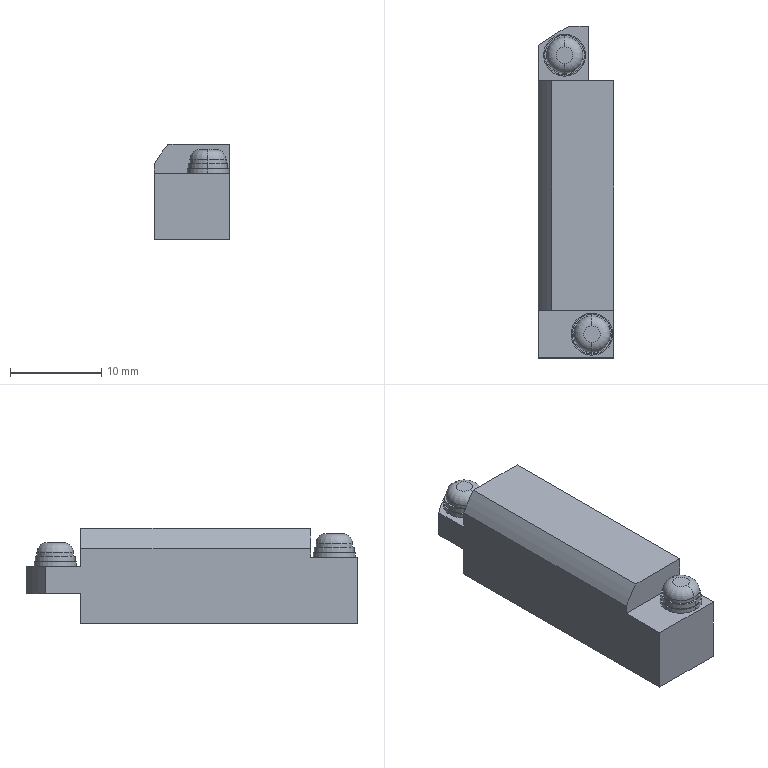Part | STEP file | Guide wheel mechanism revised.sldasm-Part-33 | 1 solid | 36 faces | box 8.3 x 36.4 x 10.5 mm | volume 2626 mm3 | plane 18 | cylinder 14 | torus 4 | commonest cylinder face diameters 4 x4 4.35 x4 4.6 x4 32 x1 47 x1
STEP:
#1=CARTESIAN_POINT('',(-8.1,318.9,-3.2));
#2=VERTEX_POINT('',#1);
#3=CARTESIAN_POINT('',(-8.1,323.5,-3.2));
#4=VERTEX_POINT('',#3);
#5=CARTESIAN_POINT('',(-8.1,321.2,-3.2));
#6=DIRECTION('',(0.,0.,1.));
#7=DIRECTION('',(0.,-1.,0.));
#8=AXIS2_PLACEMENT_3D('',#5,#6,#7);
#9=CIRCLE('',#8,2.3);
#10=EDGE_CURVE('',#2,#4,#9,.T.);
#11=ORIENTED_EDGE('',*,*,#10,.T.);
#12=CARTESIAN_POINT('',(-8.1,323.5,-2.7));
#13=VERTEX_POINT('',#12);
#14=CARTESIAN_POINT('',(-8.1,323.5,-0.6));
#15=DIRECTION('',(0.,0.,1.));
#16=VECTOR('',#15,1000.);
#17=LINE('',#14,#16);
#18=EDGE_CURVE('',#4,#13,#17,.T.);
#19=ORIENTED_EDGE('',*,*,#18,.T.);
#20=CARTESIAN_POINT('',(-8.1,318.9,-2.7));
#21=VERTEX_POINT('',#20);
#22=CARTESIAN_POINT('',(-8.1,321.2,-2.7));
#23=DIRECTION('',(0.,0.,-1.));
#24=DIRECTION('',(0.,-1.,0.));
#25=AXIS2_PLACEMENT_3D('',#22,#23,#24);
#26=CIRCLE('',#25,2.3);
#27=EDGE_CURVE('',#13,#21,#26,.T.);
#28=ORIENTED_EDGE('',*,*,#27,.T.);
#29=CARTESIAN_POINT('',(-8.1,318.9,-0.6));
#30=DIRECTION('',(0.,0.,1.));
#31=VECTOR('',#30,1000.);
#32=LINE('',#29,#31);
#33=EDGE_CURVE('',#2,#21,#32,.T.);
#34=ORIENTED_EDGE('',*,*,#33,.F.);
#35=EDGE_LOOP('',(#11,#19,#28,#34));
#36=FACE_OUTER_BOUND('',#35,.T.);
#37=CARTESIAN_POINT('',(-8.1,321.2,-0.6));
#38=DIRECTION('',(0.,0.,1.));
#39=DIRECTION('',(0.,-1.,0.));
#40=AXIS2_PLACEMENT_3D('',#37,#38,#39);
#41=CYLINDRICAL_SURFACE('',#40,2.3);
#42=ADVANCED_FACE('',(#36),#41,.T.);
#43=CARTESIAN_POINT('',(-11.1,354.1,-4.2));
#44=VERTEX_POINT('',#43);
#45=CARTESIAN_POINT('',(-11.1,349.5,-4.2));
#46=VERTEX_POINT('',#45);
#47=CARTESIAN_POINT('',(-11.1,351.8,-4.2));
#48=DIRECTION('',(0.,0.,-1.));
#49=DIRECTION('',(0.,-1.,0.));
#50=AXIS2_PLACEMENT_3D('',#47,#48,#49);
#51=CIRCLE('',#50,2.3);
#52=EDGE_CURVE('',#44,#46,#51,.T.);
#53=ORIENTED_EDGE('',*,*,#52,.F.);
#54=CARTESIAN_POINT('',(-11.1,354.1,-3.7));
#55=VERTEX_POINT('',#54);
#56=CARTESIAN_POINT('',(-11.1,354.1,-1.6));
#57=DIRECTION('',(0.,0.,1.));
#58=VECTOR('',#57,1000.);
#59=LINE('',#56,#58);
#60=EDGE_CURVE('',#44,#55,#59,.T.);
#61=ORIENTED_EDGE('',*,*,#60,.T.);
#62=CARTESIAN_POINT('',(-11.1,349.5,-3.7));
#63=VERTEX_POINT('',#62);
#64=CARTESIAN_POINT('',(-11.1,351.8,-3.7));
#65=DIRECTION('',(0.,0.,-1.));
#66=DIRECTION('',(0.,-1.,0.));
#67=AXIS2_PLACEMENT_3D('',#64,#65,#66);
#68=CIRCLE('',#67,2.3);
#69=EDGE_CURVE('',#55,#63,#68,.T.);
#70=ORIENTED_EDGE('',*,*,#69,.T.);
#71=CARTESIAN_POINT('',(-11.1,349.5,-1.6));
#72=DIRECTION('',(0.,0.,1.));
#73=VECTOR('',#72,1000.);
#74=LINE('',#71,#73);
#75=EDGE_CURVE('',#46,#63,#74,.T.);
#76=ORIENTED_EDGE('',*,*,#75,.F.);
#77=EDGE_LOOP('',(#53,#61,#70,#76));
#78=FACE_OUTER_BOUND('',#77,.T.);
#79=CARTESIAN_POINT('',(-11.1,351.8,-1.6));
#80=DIRECTION('',(0.,0.,1.));
#81=DIRECTION('',(0.,-1.,0.));
#82=AXIS2_PLACEMENT_3D('',#79,#80,#81);
#83=CYLINDRICAL_SURFACE('',#82,2.3);
#84=ADVANCED_FACE('',(#78),#83,.T.);
#85=CARTESIAN_POINT('',(-8.1,323.375,-2.7));
#86=VERTEX_POINT('',#85);
#87=CARTESIAN_POINT('',(-8.1,319.025,-2.7));
#88=VERTEX_POINT('',#87);
#89=CARTESIAN_POINT('',(-8.1,321.2,-2.7));
#90=DIRECTION('',(0.,0.,-1.));
#91=DIRECTION('',(0.,-1.,0.));
#92=AXIS2_PLACEMENT_3D('',#89,#90,#91);
#93=CIRCLE('',#92,2.175);
#94=EDGE_CURVE('',#86,#88,#93,.T.);
#95=ORIENTED_EDGE('',*,*,#94,.F.);
#96=CARTESIAN_POINT('',(-8.1,323.375,-2.1));
#97=VERTEX_POINT('',#96);
#98=CARTESIAN_POINT('',(-8.1,323.375,-0.6));
#99=DIRECTION('',(0.,0.,1.));
#100=VECTOR('',#99,1000.);
#101=LINE('',#98,#100);
#102=EDGE_CURVE('',#86,#97,#101,.T.);
#103=ORIENTED_EDGE('',*,*,#102,.T.);
#104=CARTESIAN_POINT('',(-8.1,319.025,-2.1));
#105=VERTEX_POINT('',#104);
#106=CARTESIAN_POINT('',(-8.1,321.2,-2.1));
#107=DIRECTION('',(0.,0.,-1.));
#108=DIRECTION('',(0.,-1.,0.));
#109=AXIS2_PLACEMENT_3D('',#106,#107,#108);
#110=CIRCLE('',#109,2.175);
#111=EDGE_CURVE('',#97,#105,#110,.T.);
#112=ORIENTED_EDGE('',*,*,#111,.T.);
#113=CARTESIAN_POINT('',(-8.1,319.025,-0.6));
#114=DIRECTION('',(0.,0.,1.));
#115=VECTOR('',#114,1000.);
#116=LINE('',#113,#115);
#117=EDGE_CURVE('',#88,#105,#116,.T.);
#118=ORIENTED_EDGE('',*,*,#117,.F.);
#119=EDGE_LOOP('',(#95,#103,#112,#118));
#120=FACE_OUTER_BOUND('',#119,.T.);
#121=CARTESIAN_POINT('',(-8.1,321.2,-0.6));
#122=DIRECTION('',(0.,0.,1.));
#123=DIRECTION('',(0.,-1.,0.));
#124=AXIS2_PLACEMENT_3D('',#121,#122,#123);
#125=CYLINDRICAL_SURFACE('',#124,2.175);
#126=ADVANCED_FACE('',(#120),#125,.T.);
#127=CARTESIAN_POINT('',(-11.1,349.625,-3.7));
#128=VERTEX_POINT('',#127);
#129=CARTESIAN_POINT('',(-11.1,353.975,-3.7));
#130=VERTEX_POINT('',#129);
#131=CARTESIAN_POINT('',(-11.1,351.8,-3.7));
#132=DIRECTION('',(0.,0.,1.));
#133=DIRECTION('',(0.,-1.,0.));
#134=AXIS2_PLACEMENT_3D('',#131,#132,#133);
#135=CIRCLE('',#134,2.175);
#136=EDGE_CURVE('',#128,#130,#135,.T.);
#137=ORIENTED_EDGE('',*,*,#136,.T.);
#138=CARTESIAN_POINT('',(-11.1,353.975,-3.1));
#139=VERTEX_POINT('',#138);
#140=CARTESIAN_POINT('',(-11.1,353.975,-1.6));
#141=DIRECTION('',(0.,0.,1.));
#142=VECTOR('',#141,1000.);
#143=LINE('',#140,#142);
#144=EDGE_CURVE('',#130,#139,#143,.T.);
#145=ORIENTED_EDGE('',*,*,#144,.T.);
#146=CARTESIAN_POINT('',(-11.1,349.625,-3.1));
#147=VERTEX_POINT('',#146);
#148=CARTESIAN_POINT('',(-11.1,351.8,-3.1));
#149=DIRECTION('',(0.,0.,-1.));
#150=DIRECTION('',(0.,-1.,0.));
#151=AXIS2_PLACEMENT_3D('',#148,#149,#150);
#152=CIRCLE('',#151,2.175);
#153=EDGE_CURVE('',#139,#147,#152,.T.);
#154=ORIENTED_EDGE('',*,*,#153,.T.);
#155=CARTESIAN_POINT('',(-11.1,349.625,-1.6));
#156=DIRECTION('',(0.,0.,1.));
#157=VECTOR('',#156,1000.);
#158=LINE('',#155,#157);
#159=EDGE_CURVE('',#128,#147,#158,.T.);
#160=ORIENTED_EDGE('',*,*,#159,.F.);
#161=EDGE_LOOP('',(#137,#145,#154,#160));
#162=FACE_OUTER_BOUND('',#161,.T.);
#163=CARTESIAN_POINT('',(-11.1,351.8,-1.6));
#164=DIRECTION('',(0.,0.,1.));
#165=DIRECTION('',(0.,-1.,0.));
#166=AXIS2_PLACEMENT_3D('',#163,#164,#165);
#167=CYLINDRICAL_SURFACE('',#166,2.175);
#168=ADVANCED_FACE('',(#162),#167,.T.);
#169=CARTESIAN_POINT('',(-8.1,323.2,-2.1));
#170=VERTEX_POINT('',#169);
#171=CARTESIAN_POINT('',(-8.1,319.2,-2.1));
#172=VERTEX_POINT('',#171);
#173=CARTESIAN_POINT('',(-8.1,321.2,-2.1));
#174=DIRECTION('',(0.,0.,-1.));
#175=DIRECTION('',(0.,-1.,0.));
#176=AXIS2_PLACEMENT_3D('',#173,#174,#175);
#177=CIRCLE('',#176,2.);
#178=EDGE_CURVE('',#170,#172,#177,.T.);
#179=ORIENTED_EDGE('',*,*,#178,.F.);
#180=CARTESIAN_POINT('',(-8.1,323.2,-1.7));
#181=VERTEX_POINT('',#180);
#182=CARTESIAN_POINT('',(-8.1,323.2,-0.6));
#183=DIRECTION('',(0.,0.,1.));
#184=VECTOR('',#183,1000.);
#185=LINE('',#182,#184);
#186=EDGE_CURVE('',#170,#181,#185,.T.);
#187=ORIENTED_EDGE('',*,*,#186,.T.);
#188=CARTESIAN_POINT('',(-8.1,319.2,-1.7));
#189=VERTEX_POINT('',#188);
#190=CARTESIAN_POINT('',(-8.1,321.2,-1.7));
#191=DIRECTION('',(0.,0.,-1.));
#192=DIRECTION('',(0.,-1.,0.));
#193=AXIS2_PLACEMENT_3D('',#190,#191,#192);
#194=CIRCLE('',#193,2.);
#195=EDGE_CURVE('',#181,#189,#194,.T.);
#196=ORIENTED_EDGE('',*,*,#195,.T.);
#197=CARTESIAN_POINT('',(-8.1,319.2,-0.6));
#198=DIRECTION('',(0.,0.,1.));
#199=VECTOR('',#198,1000.);
#200=LINE('',#197,#199);
#201=EDGE_CURVE('',#172,#189,#200,.T.);
#202=ORIENTED_EDGE('',*,*,#201,.F.);
#203=EDGE_LOOP('',(#179,#187,#196,#202));
#204=FACE_OUTER_BOUND('',#203,.T.);
#205=CARTESIAN_POINT('',(-8.1,321.2,-0.6));
#206=DIRECTION('',(0.,0.,1.));
#207=DIRECTION('',(0.,-1.,0.));
#208=AXIS2_PLACEMENT_3D('',#205,#206,#207);
#209=CYLINDRICAL_SURFACE('',#208,2.);
#210=ADVANCED_FACE('',(#204),#209,.T.);
#211=CARTESIAN_POINT('',(-11.1,349.8,-3.1));
#212=VERTEX_POINT('',#211);
#213=CARTESIAN_POINT('',(-11.1,353.8,-3.1));
#214=VERTEX_POINT('',#213);
#215=CARTESIAN_POINT('',(-11.1,351.8,-3.1));
#216=DIRECTION('',(0.,0.,1.));
#217=DIRECTION('',(0.,-1.,0.));
#218=AXIS2_PLACEMENT_3D('',#215,#216,#217);
#219=CIRCLE('',#218,2.);
#220=EDGE_CURVE('',#212,#214,#219,.T.);
#221=ORIENTED_EDGE('',*,*,#220,.T.);
#222=CARTESIAN_POINT('',(-11.1,353.8,-2.7));
#223=VERTEX_POINT('',#222);
#224=CARTESIAN_POINT('',(-11.1,353.8,-1.6));
#225=DIRECTION('',(0.,0.,1.));
#226=VECTOR('',#225,1000.);
#227=LINE('',#224,#226);
#228=EDGE_CURVE('',#214,#223,#227,.T.);
#229=ORIENTED_EDGE('',*,*,#228,.T.);
#230=CARTESIAN_POINT('',(-11.1,349.8,-2.7));
#231=VERTEX_POINT('',#230);
#232=CARTESIAN_POINT('',(-11.1,351.8,-2.7));
#233=DIRECTION('',(0.,0.,-1.));
#234=DIRECTION('',(0.,-1.,0.));
#235=AXIS2_PLACEMENT_3D('',#232,#233,#234);
#236=CIRCLE('',#235,2.);
#237=EDGE_CURVE('',#223,#231,#236,.T.);
#238=ORIENTED_EDGE('',*,*,#237,.T.);
#239=CARTESIAN_POINT('',(-11.1,349.8,-1.6));
#240=DIRECTION('',(0.,0.,1.));
#241=VECTOR('',#240,1000.);
#242=LINE('',#239,#241);
#243=EDGE_CURVE('',#212,#231,#242,.T.);
#244=ORIENTED_EDGE('',*,*,#243,.F.);
#245=EDGE_LOOP('',(#221,#229,#238,#244));
#246=FACE_OUTER_BOUND('',#245,.T.);
#247=CARTESIAN_POINT('',(-11.1,351.8,-1.6));
#248=DIRECTION('',(0.,0.,1.));
#249=DIRECTION('',(0.,-1.,0.));
#250=AXIS2_PLACEMENT_3D('',#247,#248,#249);
#251=CYLINDRICAL_SURFACE('',#250,2.);
#252=ADVANCED_FACE('',(#246),#251,.T.);
#253=ORIENTED_EDGE('',*,*,#195,.F.);
#254=CARTESIAN_POINT('',(-8.1,322.1,-0.6));
#255=VERTEX_POINT('',#254);
#256=CARTESIAN_POINT('',(-8.1,322.1,-1.7));
#257=DIRECTION('',(1.,0.,0.));
#258=DIRECTION('',(0.,1.,0.));
#259=AXIS2_PLACEMENT_3D('',#256,#257,#258);
#260=CIRCLE('',#259,1.1);
#261=EDGE_CURVE('',#181,#255,#260,.T.);
#262=ORIENTED_EDGE('',*,*,#261,.T.);
#263=CARTESIAN_POINT('',(-8.1,320.3,-0.6));
#264=VERTEX_POINT('',#263);
#265=CARTESIAN_POINT('',(-8.1,321.2,-0.6));
#266=DIRECTION('',(0.,0.,-1.));
#267=DIRECTION('',(0.,-1.,0.));
#268=AXIS2_PLACEMENT_3D('',#265,#266,#267);
#269=CIRCLE('',#268,0.9);
#270=EDGE_CURVE('',#255,#264,#269,.T.);
#271=ORIENTED_EDGE('',*,*,#270,.T.);
#272=CARTESIAN_POINT('',(-8.1,320.3,-1.7));
#273=DIRECTION('',(-1.,0.,0.));
#274=DIRECTION('',(0.,0.,1.));
#275=AXIS2_PLACEMENT_3D('',#272,#273,#274);
#276=CIRCLE('',#275,1.1);
#277=EDGE_CURVE('',#189,#264,#276,.T.);
#278=ORIENTED_EDGE('',*,*,#277,.F.);
#279=EDGE_LOOP('',(#253,#262,#271,#278));
#280=FACE_OUTER_BOUND('',#279,.T.);
#281=CARTESIAN_POINT('',(-8.1,321.2,-1.7));
#282=DIRECTION('',(0.,0.,1.));
#283=DIRECTION('',(0.,-1.,0.));
#284=AXIS2_PLACEMENT_3D('',#281,#282,#283);
#285=TOROIDAL_SURFACE('',#284,0.9,1.1);
#286=ADVANCED_FACE('',(#280),#285,.T.);
#287=ORIENTED_EDGE('',*,*,#237,.F.);
#288=CARTESIAN_POINT('',(-11.1,352.7,-1.6));
#289=VERTEX_POINT('',#288);
#290=CARTESIAN_POINT('',(-11.1,352.7,-2.7));
#291=DIRECTION('',(1.,0.,0.));
#292=DIRECTION('',(0.,1.,0.));
#293=AXIS2_PLACEMENT_3D('',#290,#291,#292);
#294=CIRCLE('',#293,1.1);
#295=EDGE_CURVE('',#223,#289,#294,.T.);
#296=ORIENTED_EDGE('',*,*,#295,.T.);
#297=CARTESIAN_POINT('',(-11.1,350.9,-1.6));
#298=VERTEX_POINT('',#297);
#299=CARTESIAN_POINT('',(-11.1,351.8,-1.6));
#300=DIRECTION('',(0.,0.,-1.));
#301=DIRECTION('',(0.,-1.,0.));
#302=AXIS2_PLACEMENT_3D('',#299,#300,#301);
#303=CIRCLE('',#302,0.9);
#304=EDGE_CURVE('',#289,#298,#303,.T.);
#305=ORIENTED_EDGE('',*,*,#304,.T.);
#306=CARTESIAN_POINT('',(-11.1,350.9,-2.7));
#307=DIRECTION('',(-1.,0.,0.));
#308=DIRECTION('',(0.,0.,1.));
#309=AXIS2_PLACEMENT_3D('',#306,#307,#308);
#310=CIRCLE('',#309,1.1);
#311=EDGE_CURVE('',#231,#298,#310,.T.);
#312=ORIENTED_EDGE('',*,*,#311,.F.);
#313=EDGE_LOOP('',(#287,#296,#305,#312));
#314=FACE_OUTER_BOUND('',#313,.T.);
#315=CARTESIAN_POINT('',(-11.1,351.8,-2.7));
#316=DIRECTION('',(0.,0.,1.));
#317=DIRECTION('',(0.,-1.,0.));
#318=AXIS2_PLACEMENT_3D('',#315,#316,#317);
#319=TOROIDAL_SURFACE('',#318,0.9,1.1);
#320=ADVANCED_FACE('',(#314),#319,.T.);
#321=CARTESIAN_POINT('',(-5.7,349.,0.));
#322=VERTEX_POINT('',#321);
#323=CARTESIAN_POINT('',(-5.7,349.,-10.5));
#324=VERTEX_POINT('',#323);
#325=CARTESIAN_POINT('',(-5.7,349.,0.));
#326=DIRECTION('',(0.,0.,-1.));
#327=VECTOR('',#326,1000.);
#328=LINE('',#325,#327);
#329=EDGE_CURVE('',#322,#324,#328,.T.);
#330=ORIENTED_EDGE('',*,*,#329,.F.);
#331=CARTESIAN_POINT('',(-5.7,323.8,0.));
#332=VERTEX_POINT('',#331);
#333=CARTESIAN_POINT('',(-5.7,323.8,0.));
#334=DIRECTION('',(0.,1.,0.));
#335=VECTOR('',#334,1000.);
#336=LINE('',#333,#335);
#337=EDGE_CURVE('',#332,#322,#336,.T.);
#338=ORIENTED_EDGE('',*,*,#337,.F.);
#339=CARTESIAN_POINT('',(-5.7,323.8,-3.2));
#340=VERTEX_POINT('',#339);
#341=CARTESIAN_POINT('',(-5.7,323.8,0.));
#342=DIRECTION('',(0.,0.,1.));
#343=VECTOR('',#342,1000.);
#344=LINE('',#341,#343);
#345=EDGE_CURVE('',#340,#332,#344,.T.);
#346=ORIENTED_EDGE('',*,*,#345,.F.);
#347=CARTESIAN_POINT('',(-5.7,318.6,-3.2));
#348=VERTEX_POINT('',#347);
#349=CARTESIAN_POINT('',(-5.7,323.8,-3.2));
#350=DIRECTION('',(0.,1.,0.));
#351=VECTOR('',#350,1000.);
#352=LINE('',#349,#351);
#353=EDGE_CURVE('',#348,#340,#352,.T.);
#354=ORIENTED_EDGE('',*,*,#353,.F.);
#355=CARTESIAN_POINT('',(-5.7,318.6,-10.5));
#356=VERTEX_POINT('',#355);
#357=CARTESIAN_POINT('',(-5.7,318.6,0.));
#358=DIRECTION('',(0.,0.,1.));
#359=VECTOR('',#358,1000.);
#360=LINE('',#357,#359);
#361=EDGE_CURVE('',#356,#348,#360,.T.);
#362=ORIENTED_EDGE('',*,*,#361,.F.);
#363=CARTESIAN_POINT('',(-5.7,323.8,-10.5));
#364=DIRECTION('',(0.,-1.,0.));
#365=VECTOR('',#364,1000.);
#366=LINE('',#363,#365);
#367=EDGE_CURVE('',#324,#356,#366,.T.);
#368=ORIENTED_EDGE('',*,*,#367,.F.);
#369=EDGE_LOOP('',(#330,#338,#346,#354,#362,#368));
#370=FACE_OUTER_BOUND('',#369,.T.);
#371=CARTESIAN_POINT('',(-5.7,323.8,0.));
#372=DIRECTION('',(-1.,0.,0.));
#373=DIRECTION('',(0.,0.,1.));
#374=AXIS2_PLACEMENT_3D('',#371,#372,#373);
#375=PLANE('',#374);
#376=ADVANCED_FACE('',(#370),#375,.F.);
#377=CARTESIAN_POINT('',(-14.,318.6,-10.5));
#378=VERTEX_POINT('',#377);
#379=CARTESIAN_POINT('',(-8.5,318.6,-10.5));
#380=DIRECTION('',(1.,0.,0.));
#381=VECTOR('',#380,1000.);
#382=LINE('',#379,#381);
#383=EDGE_CURVE('',#378,#356,#382,.T.);
#384=ORIENTED_EDGE('',*,*,#383,.F.);
#385=CARTESIAN_POINT('',(-14.,349.,-10.5));
#386=VERTEX_POINT('',#385);
#387=CARTESIAN_POINT('',(-14.,343.462,-10.5));
#388=DIRECTION('',(0.,-1.,0.));
#389=VECTOR('',#388,1000.);
#390=LINE('',#387,#389);
#391=EDGE_CURVE('',#386,#378,#390,.T.);
#392=ORIENTED_EDGE('',*,*,#391,.F.);
#393=CARTESIAN_POINT('',(-8.5,349.,-10.5));
#394=DIRECTION('',(-1.,0.,0.));
#395=VECTOR('',#394,1000.);
#396=LINE('',#393,#395);
#397=EDGE_CURVE('',#324,#386,#396,.T.);
#398=ORIENTED_EDGE('',*,*,#397,.F.);
#399=ORIENTED_EDGE('',*,*,#367,.T.);
#400=EDGE_LOOP('',(#384,#392,#398,#399));
#401=FACE_OUTER_BOUND('',#400,.T.);
#402=CARTESIAN_POINT('',(-8.5,343.462,-10.5));
#403=DIRECTION('',(0.,0.,1.));
#404=DIRECTION('',(0.,-1.,0.));
#405=AXIS2_PLACEMENT_3D('',#402,#403,#404);
#406=PLANE('',#405);
#407=ADVANCED_FACE('',(#401),#406,.F.);
#408=CARTESIAN_POINT('',(-14.,349.,-4.2));
#409=VERTEX_POINT('',#408);
#410=CARTESIAN_POINT('',(-14.,349.,-2.254));
#411=VERTEX_POINT('',#410);
#412=CARTESIAN_POINT('',(-14.,349.,0.));
#413=DIRECTION('',(0.,0.,1.));
#414=VECTOR('',#413,1000.);
#415=LINE('',#412,#414);
#416=EDGE_CURVE('',#409,#411,#415,.T.);
#417=ORIENTED_EDGE('',*,*,#416,.T.);
#418=CARTESIAN_POINT('',(-12.49,349.,0.));
#419=VERTEX_POINT('',#418);
#420=CARTESIAN_POINT('',(0.,349.,-10.));
#421=DIRECTION('',(0.,1.,0.));
#422=DIRECTION('',(0.,0.,1.));
#423=AXIS2_PLACEMENT_3D('',#420,#421,#422);
#424=CIRCLE('',#423,16.);
#425=EDGE_CURVE('',#411,#419,#424,.T.);
#426=ORIENTED_EDGE('',*,*,#425,.T.);
#427=CARTESIAN_POINT('',(-8.5,349.,0.));
#428=DIRECTION('',(1.,0.,0.));
#429=VECTOR('',#428,1000.);
#430=LINE('',#427,#429);
#431=EDGE_CURVE('',#419,#322,#430,.T.);
#432=ORIENTED_EDGE('',*,*,#431,.T.);
#433=ORIENTED_EDGE('',*,*,#329,.T.);
#434=ORIENTED_EDGE('',*,*,#397,.T.);
#435=CARTESIAN_POINT('',(-14.,349.,-7.2));
#436=VERTEX_POINT('',#435);
#437=CARTESIAN_POINT('',(-14.,349.,0.));
#438=DIRECTION('',(0.,0.,1.));
#439=VECTOR('',#438,1000.);
#440=LINE('',#437,#439);
#441=EDGE_CURVE('',#386,#436,#440,.T.);
#442=ORIENTED_EDGE('',*,*,#441,.T.);
#443=CARTESIAN_POINT('',(-8.5,349.,-7.2));
#444=VERTEX_POINT('',#443);
#445=CARTESIAN_POINT('',(-8.5,349.,-7.2));
#446=DIRECTION('',(1.,0.,0.));
#447=VECTOR('',#446,1000.);
#448=LINE('',#445,#447);
#449=EDGE_CURVE('',#436,#444,#448,.T.);
#450=ORIENTED_EDGE('',*,*,#449,.T.);
#451=CARTESIAN_POINT('',(-8.5,349.,-4.2));
#452=VERTEX_POINT('',#451);
#453=CARTESIAN_POINT('',(-8.5,349.,0.));
#454=DIRECTION('',(0.,0.,1.));
#455=VECTOR('',#454,1000.);
#456=LINE('',#453,#455);
#457=EDGE_CURVE('',#444,#452,#456,.T.);
#458=ORIENTED_EDGE('',*,*,#457,.T.);
#459=CARTESIAN_POINT('',(-8.5,349.,-4.2));
#460=DIRECTION('',(-1.,0.,0.));
#461=VECTOR('',#460,1000.);
#462=LINE('',#459,#461);
#463=EDGE_CURVE('',#452,#409,#462,.T.);
#464=ORIENTED_EDGE('',*,*,#463,.T.);
#465=EDGE_LOOP('',(#417,#426,#432,#433,#434,#442,#450,#458,#464));
#466=FACE_OUTER_BOUND('',#465,.T.);
#467=CARTESIAN_POINT('',(-8.5,349.,0.));
#468=DIRECTION('',(0.,1.,0.));
#469=DIRECTION('',(0.,0.,1.));
#470=AXIS2_PLACEMENT_3D('',#467,#468,#469);
#471=PLANE('',#470);
#472=ADVANCED_FACE('',(#466),#471,.T.);
#473=CARTESIAN_POINT('',(-12.49,323.8,0.));
#474=VERTEX_POINT('',#473);
#475=CARTESIAN_POINT('',(0.000000976,323.8,0.));
#476=DIRECTION('',(-1.,0.,0.));
#477=VECTOR('',#476,1000.);
#478=LINE('',#475,#477);
#479=EDGE_CURVE('',#332,#474,#478,.T.);
#480=ORIENTED_EDGE('',*,*,#479,.F.);
#481=ORIENTED_EDGE('',*,*,#337,.T.);
#482=ORIENTED_EDGE('',*,*,#431,.F.);
#483=CARTESIAN_POINT('',(-12.49,226.,0.));
#484=DIRECTION('',(0.,1.,0.));
#485=VECTOR('',#484,1000.);
#486=LINE('',#483,#485);
#487=EDGE_CURVE('',#474,#419,#486,.T.);
#488=ORIENTED_EDGE('',*,*,#487,.F.);
#489=EDGE_LOOP('',(#480,#481,#482,#488));
#490=FACE_OUTER_BOUND('',#489,.T.);
#491=CARTESIAN_POINT('',(0.000000976,226.,0.));
#492=DIRECTION('',(0.,0.,-1.));
#493=DIRECTION('',(0.,1.,0.));
#494=AXIS2_PLACEMENT_3D('',#491,#492,#493);
#495=PLANE('',#494);
#496=ADVANCED_FACE('',(#490),#495,.F.);
#497=ORIENTED_EDGE('',*,*,#479,.T.);
#498=CARTESIAN_POINT('',(-14.,323.8,-2.254));
#499=VERTEX_POINT('',#498);
#500=CARTESIAN_POINT('',(0.,323.8,-10.));
#501=DIRECTION('',(0.,-1.,0.));
#502=DIRECTION('',(0.,0.,1.));
#503=AXIS2_PLACEMENT_3D('',#500,#501,#502);
#504=CIRCLE('',#503,16.);
#505=EDGE_CURVE('',#474,#499,#504,.T.);
#506=ORIENTED_EDGE('',*,*,#505,.T.);
#507=CARTESIAN_POINT('',(-14.,323.8,-3.2));
#508=VERTEX_POINT('',#507);
#509=CARTESIAN_POINT('',(-14.,323.8,-3.2));
#510=DIRECTION('',(0.,0.,-1.));
#511=VECTOR('',#510,1000.);
#512=LINE('',#509,#511);
#513=EDGE_CURVE('',#499,#508,#512,.T.);
#514=ORIENTED_EDGE('',*,*,#513,.T.);
#515=CARTESIAN_POINT('',(-15.123,323.8,-3.2));
#516=DIRECTION('',(1.,0.,0.));
#517=VECTOR('',#516,1000.);
#518=LINE('',#515,#517);
#519=EDGE_CURVE('',#508,#340,#518,.T.);
#520=ORIENTED_EDGE('',*,*,#519,.T.);
#521=ORIENTED_EDGE('',*,*,#345,.T.);
#522=EDGE_LOOP('',(#497,#506,#514,#520,#521));
#523=FACE_OUTER_BOUND('',#522,.T.);
#524=CARTESIAN_POINT('',(-15.123,323.8,-3.2));
#525=DIRECTION('',(0.,-1.,0.));
#526=DIRECTION('',(0.,0.,-1.));
#527=AXIS2_PLACEMENT_3D('',#524,#525,#526);
#528=PLANE('',#527);
#529=ADVANCED_FACE('',(#523),#528,.T.);
#530=ORIENTED_EDGE('',*,*,#10,.F.);
#531=CARTESIAN_POINT('',(-8.1,321.2,-3.2));
#532=DIRECTION('',(0.,0.,1.));
#533=DIRECTION('',(0.,-1.,0.));
#534=AXIS2_PLACEMENT_3D('',#531,#532,#533);
#535=CIRCLE('',#534,2.3);
#536=EDGE_CURVE('',#4,#2,#535,.T.);
#537=ORIENTED_EDGE('',*,*,#536,.F.);
#538=EDGE_LOOP('',(#530,#537));
#539=FACE_BOUND('',#538,.T.);
#540=CARTESIAN_POINT('',(-14.,318.6,-3.2));
#541=VERTEX_POINT('',#540);
#542=CARTESIAN_POINT('',(-15.123,318.6,-3.2));
#543=DIRECTION('',(-1.,0.,0.));
#544=VECTOR('',#543,1000.);
#545=LINE('',#542,#544);
#546=EDGE_CURVE('',#348,#541,#545,.T.);
#547=ORIENTED_EDGE('',*,*,#546,.F.);
#548=ORIENTED_EDGE('',*,*,#353,.T.);
#549=ORIENTED_EDGE('',*,*,#519,.F.);
#550=CARTESIAN_POINT('',(-14.,323.8,-3.2));
#551=DIRECTION('',(0.,1.,0.));
#552=VECTOR('',#551,1000.);
#553=LINE('',#550,#552);
#554=EDGE_CURVE('',#541,#508,#553,.T.);
#555=ORIENTED_EDGE('',*,*,#554,.F.);
#556=EDGE_LOOP('',(#547,#548,#549,#555));
#557=FACE_OUTER_BOUND('',#556,.T.);
#558=CARTESIAN_POINT('',(-15.123,323.8,-3.2));
#559=DIRECTION('',(0.,0.,-1.));
#560=DIRECTION('',(0.,1.,0.));
#561=AXIS2_PLACEMENT_3D('',#558,#559,#560);
#562=PLANE('',#561);
#563=ADVANCED_FACE('',(#539,#557),#562,.F.);
#564=ORIENTED_EDGE('',*,*,#361,.T.);
#565=ORIENTED_EDGE('',*,*,#546,.T.);
#566=CARTESIAN_POINT('',(-14.,318.6,-8.1));
#567=DIRECTION('',(0.,0.,-1.));
#568=VECTOR('',#567,1000.);
#569=LINE('',#566,#568);
#570=EDGE_CURVE('',#541,#378,#569,.T.);
#571=ORIENTED_EDGE('',*,*,#570,.T.);
#572=ORIENTED_EDGE('',*,*,#383,.T.);
#573=EDGE_LOOP('',(#564,#565,#571,#572));
#574=FACE_OUTER_BOUND('',#573,.T.);
#575=CARTESIAN_POINT('',(-14.,318.6,-8.1));
#576=DIRECTION('',(0.,-1.,0.));
#577=DIRECTION('',(0.,0.,-1.));
#578=AXIS2_PLACEMENT_3D('',#575,#576,#577);
#579=PLANE('',#578);
#580=ADVANCED_FACE('',(#574),#579,.T.);
#581=ORIENTED_EDGE('',*,*,#570,.F.);
#582=ORIENTED_EDGE('',*,*,#554,.T.);
#583=ORIENTED_EDGE('',*,*,#513,.F.);
#584=CARTESIAN_POINT('',(-14.,207.125,-2.254));
#585=DIRECTION('',(0.,-1.,0.));
#586=VECTOR('',#585,1000.);
#587=LINE('',#584,#586);
#588=EDGE_CURVE('',#411,#499,#587,.T.);
#589=ORIENTED_EDGE('',*,*,#588,.F.);
#590=ORIENTED_EDGE('',*,*,#416,.F.);
#591=CARTESIAN_POINT('',(-14.,352.875,-4.2));
#592=VERTEX_POINT('',#591);
#593=CARTESIAN_POINT('',(-14.,207.125,-4.2));
#594=DIRECTION('',(0.,-1.,0.));
#595=VECTOR('',#594,1000.);
#596=LINE('',#593,#595);
#597=EDGE_CURVE('',#592,#409,#596,.T.);
#598=ORIENTED_EDGE('',*,*,#597,.F.);
#599=CARTESIAN_POINT('',(-14.,352.875,-7.2));
#600=VERTEX_POINT('',#599);
#601=CARTESIAN_POINT('',(-14.,352.875,-28.575));
#602=DIRECTION('',(0.,0.,1.));
#603=VECTOR('',#602,1000.);
#604=LINE('',#601,#603);
#605=EDGE_CURVE('',#600,#592,#604,.T.);
#606=ORIENTED_EDGE('',*,*,#605,.F.);
#607=CARTESIAN_POINT('',(-14.,207.125,-7.2));
#608=DIRECTION('',(0.,1.,0.));
#609=VECTOR('',#608,1000.);
#610=LINE('',#607,#609);
#611=EDGE_CURVE('',#436,#600,#610,.T.);
#612=ORIENTED_EDGE('',*,*,#611,.F.);
#613=ORIENTED_EDGE('',*,*,#441,.F.);
#614=ORIENTED_EDGE('',*,*,#391,.T.);
#615=EDGE_LOOP('',(#581,#582,#583,#589,#590,#598,#606,#612,#613,#614));
#616=FACE_OUTER_BOUND('',#615,.T.);
#617=CARTESIAN_POINT('',(-14.,207.125,-28.575));
#618=DIRECTION('',(1.,0.,0.));
#619=DIRECTION('',(0.,1.,0.));
#620=AXIS2_PLACEMENT_3D('',#617,#618,#619);
#621=PLANE('',#620);
#622=ADVANCED_FACE('',(#616),#621,.F.);
#623=ORIENTED_EDGE('',*,*,#487,.T.);
#624=ORIENTED_EDGE('',*,*,#425,.F.);
#625=ORIENTED_EDGE('',*,*,#588,.T.);
#626=ORIENTED_EDGE('',*,*,#505,.F.);
#627=EDGE_LOOP('',(#623,#624,#625,#626));
#628=FACE_OUTER_BOUND('',#627,.T.);
#629=CARTESIAN_POINT('',(0.,200.21,-10.));
#630=DIRECTION('',(0.,1.,0.));
#631=DIRECTION('',(0.,0.,1.));
#632=AXIS2_PLACEMENT_3D('',#629,#630,#631);
#633=CYLINDRICAL_SURFACE('',#632,16.);
#634=ADVANCED_FACE('',(#628),#633,.T.);
#635=CARTESIAN_POINT('',(-10.548,355.,-4.2));
#636=VERTEX_POINT('',#635);
#637=CARTESIAN_POINT('',(0.,334.,-4.2));
#638=DIRECTION('',(0.,0.,1.));
#639=DIRECTION('',(0.,-1.,0.));
#640=AXIS2_PLACEMENT_3D('',#637,#638,#639);
#641=CIRCLE('',#640,23.5);
#642=EDGE_CURVE('',#636,#592,#641,.T.);
#643=ORIENTED_EDGE('',*,*,#642,.T.);
#644=ORIENTED_EDGE('',*,*,#597,.T.);
#645=ORIENTED_EDGE('',*,*,#463,.F.);
#646=CARTESIAN_POINT('',(-8.5,355.,-4.2));
#647=VERTEX_POINT('',#646);
#648=CARTESIAN_POINT('',(-8.5,356.499,-4.2));
#649=DIRECTION('',(0.,1.,0.));
#650=VECTOR('',#649,1000.);
#651=LINE('',#648,#650);
#652=EDGE_CURVE('',#452,#647,#651,.T.);
#653=ORIENTED_EDGE('',*,*,#652,.T.);
#654=CARTESIAN_POINT('',(-15.049,355.,-4.2));
#655=DIRECTION('',(-1.,0.,0.));
#656=VECTOR('',#655,1000.);
#657=LINE('',#654,#656);
#658=EDGE_CURVE('',#647,#636,#657,.T.);
#659=ORIENTED_EDGE('',*,*,#658,.T.);
#660=EDGE_LOOP('',(#643,#644,#645,#653,#659));
#661=FACE_OUTER_BOUND('',#660,.T.);
#662=CARTESIAN_POINT('',(-11.1,351.8,-4.2));
#663=DIRECTION('',(0.,0.,-1.));
#664=DIRECTION('',(0.,-1.,0.));
#665=AXIS2_PLACEMENT_3D('',#662,#663,#664);
#666=CIRCLE('',#665,2.3);
#667=EDGE_CURVE('',#46,#44,#666,.T.);
#668=ORIENTED_EDGE('',*,*,#667,.T.);
#669=ORIENTED_EDGE('',*,*,#52,.T.);
#670=EDGE_LOOP('',(#668,#669));
#671=FACE_BOUND('',#670,.T.);
#672=CARTESIAN_POINT('',(-15.049,356.499,-4.2));
#673=DIRECTION('',(0.,0.,1.));
#674=DIRECTION('',(0.,-1.,0.));
#675=AXIS2_PLACEMENT_3D('',#672,#673,#674);
#676=PLANE('',#675);
#677=ADVANCED_FACE('',(#661,#671),#676,.T.);
#678=ORIENTED_EDGE('',*,*,#652,.F.);
#679=ORIENTED_EDGE('',*,*,#457,.F.);
#680=CARTESIAN_POINT('',(-8.5,355.,-7.2));
#681=VERTEX_POINT('',#680);
#682=CARTESIAN_POINT('',(-8.5,349.,-7.2));
#683=DIRECTION('',(0.,-1.,0.));
#684=VECTOR('',#683,1000.);
#685=LINE('',#682,#684);
#686=EDGE_CURVE('',#681,#444,#685,.T.);
#687=ORIENTED_EDGE('',*,*,#686,.F.);
#688=CARTESIAN_POINT('',(-8.5,355.,0.));
#689=DIRECTION('',(0.,0.,-1.));
#690=VECTOR('',#689,1000.);
#691=LINE('',#688,#690);
#692=EDGE_CURVE('',#647,#681,#691,.T.);
#693=ORIENTED_EDGE('',*,*,#692,.F.);
#694=EDGE_LOOP('',(#678,#679,#687,#693));
#695=FACE_OUTER_BOUND('',#694,.T.);
#696=CARTESIAN_POINT('',(-8.5,349.,0.));
#697=DIRECTION('',(-1.,0.,0.));
#698=DIRECTION('',(0.,0.,1.));
#699=AXIS2_PLACEMENT_3D('',#696,#697,#698);
#700=PLANE('',#699);
#701=ADVANCED_FACE('',(#695),#700,.F.);
#702=CARTESIAN_POINT('',(-10.548,355.,-7.2));
#703=VERTEX_POINT('',#702);
#704=CARTESIAN_POINT('',(0.,334.,-7.2));
#705=DIRECTION('',(0.,0.,1.));
#706=DIRECTION('',(0.,-1.,0.));
#707=AXIS2_PLACEMENT_3D('',#704,#705,#706);
#708=CIRCLE('',#707,23.5);
#709=EDGE_CURVE('',#703,#600,#708,.T.);
#710=ORIENTED_EDGE('',*,*,#709,.F.);
#711=CARTESIAN_POINT('',(-10.548,355.,-7.2));
#712=DIRECTION('',(-1.,0.,0.));
#713=VECTOR('',#712,1000.);
#714=LINE('',#711,#713);
#715=EDGE_CURVE('',#681,#703,#714,.T.);
#716=ORIENTED_EDGE('',*,*,#715,.F.);
#717=ORIENTED_EDGE('',*,*,#686,.T.);
#718=ORIENTED_EDGE('',*,*,#449,.F.);
#719=ORIENTED_EDGE('',*,*,#611,.T.);
#720=EDGE_LOOP('',(#710,#716,#717,#718,#719));
#721=FACE_OUTER_BOUND('',#720,.T.);
#722=CARTESIAN_POINT('',(-10.548,355.,-7.2));
#723=DIRECTION('',(0.,0.,1.));
#724=DIRECTION('',(0.,-1.,0.));
#725=AXIS2_PLACEMENT_3D('',#722,#723,#724);
#726=PLANE('',#725);
#727=ADVANCED_FACE('',(#721),#726,.F.);
#728=ORIENTED_EDGE('',*,*,#18,.F.);
#729=ORIENTED_EDGE('',*,*,#536,.T.);
#730=ORIENTED_EDGE('',*,*,#33,.T.);
#731=CARTESIAN_POINT('',(-8.1,321.2,-2.7));
#732=DIRECTION('',(0.,0.,-1.));
#733=DIRECTION('',(0.,-1.,0.));
#734=AXIS2_PLACEMENT_3D('',#731,#732,#733);
#735=CIRCLE('',#734,2.3);
#736=EDGE_CURVE('',#21,#13,#735,.T.);
#737=ORIENTED_EDGE('',*,*,#736,.T.);
#738=EDGE_LOOP('',(#728,#729,#730,#737));
#739=FACE_OUTER_BOUND('',#738,.T.);
#740=CARTESIAN_POINT('',(-8.1,321.2,-0.6));
#741=DIRECTION('',(0.,0.,1.));
#742=DIRECTION('',(0.,-1.,0.));
#743=AXIS2_PLACEMENT_3D('',#740,#741,#742);
#744=CYLINDRICAL_SURFACE('',#743,2.3);
#745=ADVANCED_FACE('',(#739),#744,.T.);
#746=CARTESIAN_POINT('',(-10.548,355.,-28.575));
#747=DIRECTION('',(0.,0.,-1.));
#748=VECTOR('',#747,1000.);
#749=LINE('',#746,#748);
#750=EDGE_CURVE('',#636,#703,#749,.T.);
#751=ORIENTED_EDGE('',*,*,#750,.T.);
#752=ORIENTED_EDGE('',*,*,#709,.T.);
#753=ORIENTED_EDGE('',*,*,#605,.T.);
#754=ORIENTED_EDGE('',*,*,#642,.F.);
#755=EDGE_LOOP('',(#751,#752,#753,#754));
#756=FACE_OUTER_BOUND('',#755,.T.);
#757=CARTESIAN_POINT('',(0.,334.,-28.575));
#758=DIRECTION('',(0.,0.,1.));
#759=DIRECTION('',(0.,-1.,0.));
#760=AXIS2_PLACEMENT_3D('',#757,#758,#759);
#761=CYLINDRICAL_SURFACE('',#760,23.5);
#762=ADVANCED_FACE('',(#756),#761,.T.);
#763=ORIENTED_EDGE('',*,*,#658,.F.);
#764=ORIENTED_EDGE('',*,*,#692,.T.);
#765=ORIENTED_EDGE('',*,*,#715,.T.);
#766=ORIENTED_EDGE('',*,*,#750,.F.);
#767=EDGE_LOOP('',(#763,#764,#765,#766));
#768=FACE_OUTER_BOUND('',#767,.T.);
#769=CARTESIAN_POINT('',(10.548,355.,-28.575));
#770=DIRECTION('',(0.,-1.,0.));
#771=DIRECTION('',(0.,0.,-1.));
#772=AXIS2_PLACEMENT_3D('',#769,#770,#771);
#773=PLANE('',#772);
#774=ADVANCED_FACE('',(#768),#773,.F.);
#775=ORIENTED_EDGE('',*,*,#60,.F.);
#776=ORIENTED_EDGE('',*,*,#667,.F.);
#777=ORIENTED_EDGE('',*,*,#75,.T.);
#778=CARTESIAN_POINT('',(-11.1,351.8,-3.7));
#779=DIRECTION('',(0.,0.,-1.));
#780=DIRECTION('',(0.,-1.,0.));
#781=AXIS2_PLACEMENT_3D('',#778,#779,#780);
#782=CIRCLE('',#781,2.3);
#783=EDGE_CURVE('',#63,#55,#782,.T.);
#784=ORIENTED_EDGE('',*,*,#783,.T.);
#785=EDGE_LOOP('',(#775,#776,#777,#784));
#786=FACE_OUTER_BOUND('',#785,.T.);
#787=CARTESIAN_POINT('',(-11.1,351.8,-1.6));
#788=DIRECTION('',(0.,0.,1.));
#789=DIRECTION('',(0.,-1.,0.));
#790=AXIS2_PLACEMENT_3D('',#787,#788,#789);
#791=CYLINDRICAL_SURFACE('',#790,2.3);
#792=ADVANCED_FACE('',(#786),#791,.T.);
#793=CARTESIAN_POINT('',(-8.1,321.2,-2.7));
#794=DIRECTION('',(0.,0.,-1.));
#795=DIRECTION('',(0.,-1.,0.));
#796=AXIS2_PLACEMENT_3D('',#793,#794,#795);
#797=CIRCLE('',#796,2.175);
#798=EDGE_CURVE('',#88,#86,#797,.T.);
#799=ORIENTED_EDGE('',*,*,#798,.T.);
#800=ORIENTED_EDGE('',*,*,#94,.T.);
#801=EDGE_LOOP('',(#799,#800));
#802=FACE_BOUND('',#801,.T.);
#803=ORIENTED_EDGE('',*,*,#736,.F.);
#804=ORIENTED_EDGE('',*,*,#27,.F.);
#805=EDGE_LOOP('',(#803,#804));
#806=FACE_OUTER_BOUND('',#805,.T.);
#807=CARTESIAN_POINT('',(-8.1,318.9,-2.7));
#808=DIRECTION('',(0.,0.,1.));
#809=DIRECTION('',(0.,-1.,0.));
#810=AXIS2_PLACEMENT_3D('',#807,#808,#809);
#811=PLANE('',#810);
#812=ADVANCED_FACE('',(#802,#806),#811,.T.);
#813=ORIENTED_EDGE('',*,*,#136,.F.);
#814=CARTESIAN_POINT('',(-11.1,351.8,-3.7));
#815=DIRECTION('',(0.,0.,1.));
#816=DIRECTION('',(0.,-1.,0.));
#817=AXIS2_PLACEMENT_3D('',#814,#815,#816);
#818=CIRCLE('',#817,2.175);
#819=EDGE_CURVE('',#130,#128,#818,.T.);
#820=ORIENTED_EDGE('',*,*,#819,.F.);
#821=EDGE_LOOP('',(#813,#820));
#822=FACE_BOUND('',#821,.T.);
#823=ORIENTED_EDGE('',*,*,#783,.F.);
#824=ORIENTED_EDGE('',*,*,#69,.F.);
#825=EDGE_LOOP('',(#823,#824));
#826=FACE_OUTER_BOUND('',#825,.T.);
#827=CARTESIAN_POINT('',(-11.1,349.5,-3.7));
#828=DIRECTION('',(0.,0.,-1.));
#829=DIRECTION('',(0.,1.,0.));
#830=AXIS2_PLACEMENT_3D('',#827,#828,#829);
#831=PLANE('',#830);
#832=ADVANCED_FACE('',(#822,#826),#831,.F.);
#833=ORIENTED_EDGE('',*,*,#102,.F.);
#834=ORIENTED_EDGE('',*,*,#798,.F.);
#835=ORIENTED_EDGE('',*,*,#117,.T.);
#836=CARTESIAN_POINT('',(-8.1,321.2,-2.1));
#837=DIRECTION('',(0.,0.,-1.));
#838=DIRECTION('',(0.,-1.,0.));
#839=AXIS2_PLACEMENT_3D('',#836,#837,#838);
#840=CIRCLE('',#839,2.175);
#841=EDGE_CURVE('',#105,#97,#840,.T.);
#842=ORIENTED_EDGE('',*,*,#841,.T.);
#843=EDGE_LOOP('',(#833,#834,#835,#842));
#844=FACE_OUTER_BOUND('',#843,.T.);
#845=CARTESIAN_POINT('',(-8.1,321.2,-0.6));
#846=DIRECTION('',(0.,0.,1.));
#847=DIRECTION('',(0.,-1.,0.));
#848=AXIS2_PLACEMENT_3D('',#845,#846,#847);
#849=CYLINDRICAL_SURFACE('',#848,2.175);
#850=ADVANCED_FACE('',(#844),#849,.T.);
#851=ORIENTED_EDGE('',*,*,#144,.F.);
#852=ORIENTED_EDGE('',*,*,#819,.T.);
#853=ORIENTED_EDGE('',*,*,#159,.T.);
#854=CARTESIAN_POINT('',(-11.1,351.8,-3.1));
#855=DIRECTION('',(0.,0.,-1.));
#856=DIRECTION('',(0.,-1.,0.));
#857=AXIS2_PLACEMENT_3D('',#854,#855,#856);
#858=CIRCLE('',#857,2.175);
#859=EDGE_CURVE('',#147,#139,#858,.T.);
#860=ORIENTED_EDGE('',*,*,#859,.T.);
#861=EDGE_LOOP('',(#851,#852,#853,#860));
#862=FACE_OUTER_BOUND('',#861,.T.);
#863=CARTESIAN_POINT('',(-11.1,351.8,-1.6));
#864=DIRECTION('',(0.,0.,1.));
#865=DIRECTION('',(0.,-1.,0.));
#866=AXIS2_PLACEMENT_3D('',#863,#864,#865);
#867=CYLINDRICAL_SURFACE('',#866,2.175);
#868=ADVANCED_FACE('',(#862),#867,.T.);
#869=CARTESIAN_POINT('',(-8.1,321.2,-2.1));
#870=DIRECTION('',(0.,0.,-1.));
#871=DIRECTION('',(0.,-1.,0.));
#872=AXIS2_PLACEMENT_3D('',#869,#870,#871);
#873=CIRCLE('',#872,2.);
#874=EDGE_CURVE('',#172,#170,#873,.T.);
#875=ORIENTED_EDGE('',*,*,#874,.T.);
#876=ORIENTED_EDGE('',*,*,#178,.T.);
#877=EDGE_LOOP('',(#875,#876));
#878=FACE_BOUND('',#877,.T.);
#879=ORIENTED_EDGE('',*,*,#841,.F.);
#880=ORIENTED_EDGE('',*,*,#111,.F.);
#881=EDGE_LOOP('',(#879,#880));
#882=FACE_OUTER_BOUND('',#881,.T.);
#883=CARTESIAN_POINT('',(-8.1,319.025,-2.1));
#884=DIRECTION('',(0.,0.,1.));
#885=DIRECTION('',(0.,-1.,0.));
#886=AXIS2_PLACEMENT_3D('',#883,#884,#885);
#887=PLANE('',#886);
#888=ADVANCED_FACE('',(#878,#882),#887,.T.);
#889=ORIENTED_EDGE('',*,*,#220,.F.);
#890=CARTESIAN_POINT('',(-11.1,351.8,-3.1));
#891=DIRECTION('',(0.,0.,1.));
#892=DIRECTION('',(0.,-1.,0.));
#893=AXIS2_PLACEMENT_3D('',#890,#891,#892);
#894=CIRCLE('',#893,2.);
#895=EDGE_CURVE('',#214,#212,#894,.T.);
#896=ORIENTED_EDGE('',*,*,#895,.F.);
#897=EDGE_LOOP('',(#889,#896));
#898=FACE_BOUND('',#897,.T.);
#899=ORIENTED_EDGE('',*,*,#859,.F.);
#900=ORIENTED_EDGE('',*,*,#153,.F.);
#901=EDGE_LOOP('',(#899,#900));
#902=FACE_OUTER_BOUND('',#901,.T.);
#903=CARTESIAN_POINT('',(-11.1,349.625,-3.1));
#904=DIRECTION('',(0.,0.,-1.));
#905=DIRECTION('',(0.,1.,0.));
#906=AXIS2_PLACEMENT_3D('',#903,#904,#905);
#907=PLANE('',#906);
#908=ADVANCED_FACE('',(#898,#902),#907,.F.);
#909=ORIENTED_EDGE('',*,*,#186,.F.);
#910=ORIENTED_EDGE('',*,*,#874,.F.);
#911=ORIENTED_EDGE('',*,*,#201,.T.);
#912=CARTESIAN_POINT('',(-8.1,321.2,-1.7));
#913=DIRECTION('',(0.,0.,-1.));
#914=DIRECTION('',(0.,-1.,0.));
#915=AXIS2_PLACEMENT_3D('',#912,#913,#914);
#916=CIRCLE('',#915,2.);
#917=EDGE_CURVE('',#189,#181,#916,.T.);
#918=ORIENTED_EDGE('',*,*,#917,.T.);
#919=EDGE_LOOP('',(#909,#910,#911,#918));
#920=FACE_OUTER_BOUND('',#919,.T.);
#921=CARTESIAN_POINT('',(-8.1,321.2,-0.6));
#922=DIRECTION('',(0.,0.,1.));
#923=DIRECTION('',(0.,-1.,0.));
#924=AXIS2_PLACEMENT_3D('',#921,#922,#923);
#925=CYLINDRICAL_SURFACE('',#924,2.);
#926=ADVANCED_FACE('',(#920),#925,.T.);
#927=ORIENTED_EDGE('',*,*,#228,.F.);
#928=ORIENTED_EDGE('',*,*,#895,.T.);
#929=ORIENTED_EDGE('',*,*,#243,.T.);
#930=CARTESIAN_POINT('',(-11.1,351.8,-2.7));
#931=DIRECTION('',(0.,0.,-1.));
#932=DIRECTION('',(0.,-1.,0.));
#933=AXIS2_PLACEMENT_3D('',#930,#931,#932);
#934=CIRCLE('',#933,2.);
#935=EDGE_CURVE('',#231,#223,#934,.T.);
#936=ORIENTED_EDGE('',*,*,#935,.T.);
#937=EDGE_LOOP('',(#927,#928,#929,#936));
#938=FACE_OUTER_BOUND('',#937,.T.);
#939=CARTESIAN_POINT('',(-11.1,351.8,-1.6));
#940=DIRECTION('',(0.,0.,1.));
#941=DIRECTION('',(0.,-1.,0.));
#942=AXIS2_PLACEMENT_3D('',#939,#940,#941);
#943=CYLINDRICAL_SURFACE('',#942,2.);
#944=ADVANCED_FACE('',(#938),#943,.T.);
#945=ORIENTED_EDGE('',*,*,#261,.F.);
#946=ORIENTED_EDGE('',*,*,#917,.F.);
#947=ORIENTED_EDGE('',*,*,#277,.T.);
#948=CARTESIAN_POINT('',(-8.1,321.2,-0.6));
#949=DIRECTION('',(0.,0.,-1.));
#950=DIRECTION('',(0.,-1.,0.));
#951=AXIS2_PLACEMENT_3D('',#948,#949,#950);
#952=CIRCLE('',#951,0.9);
#953=EDGE_CURVE('',#264,#255,#952,.T.);
#954=ORIENTED_EDGE('',*,*,#953,.T.);
#955=EDGE_LOOP('',(#945,#946,#947,#954));
#956=FACE_OUTER_BOUND('',#955,.T.);
#957=CARTESIAN_POINT('',(-8.1,321.2,-1.7));
#958=DIRECTION('',(0.,0.,1.));
#959=DIRECTION('',(0.,-1.,0.));
#960=AXIS2_PLACEMENT_3D('',#957,#958,#959);
#961=TOROIDAL_SURFACE('',#960,0.9,1.1);
#962=ADVANCED_FACE('',(#956),#961,.T.);
#963=ORIENTED_EDGE('',*,*,#295,.F.);
#964=ORIENTED_EDGE('',*,*,#935,.F.);
#965=ORIENTED_EDGE('',*,*,#311,.T.);
#966=CARTESIAN_POINT('',(-11.1,351.8,-1.6));
#967=DIRECTION('',(0.,0.,-1.));
#968=DIRECTION('',(0.,-1.,0.));
#969=AXIS2_PLACEMENT_3D('',#966,#967,#968);
#970=CIRCLE('',#969,0.9);
#971=EDGE_CURVE('',#298,#289,#970,.T.);
#972=ORIENTED_EDGE('',*,*,#971,.T.);
#973=EDGE_LOOP('',(#963,#964,#965,#972));
#974=FACE_OUTER_BOUND('',#973,.T.);
#975=CARTESIAN_POINT('',(-11.1,351.8,-2.7));
#976=DIRECTION('',(0.,0.,1.));
#977=DIRECTION('',(0.,-1.,0.));
#978=AXIS2_PLACEMENT_3D('',#975,#976,#977);
#979=TOROIDAL_SURFACE('',#978,0.9,1.1);
#980=ADVANCED_FACE('',(#974),#979,.T.);
#981=ORIENTED_EDGE('',*,*,#953,.F.);
#982=ORIENTED_EDGE('',*,*,#270,.F.);
#983=EDGE_LOOP('',(#981,#982));
#984=FACE_OUTER_BOUND('',#983,.T.);
#985=CARTESIAN_POINT('',(-8.1,321.2,-0.6));
#986=DIRECTION('',(0.,0.,1.));
#987=DIRECTION('',(0.,-1.,0.));
#988=AXIS2_PLACEMENT_3D('',#985,#986,#987);
#989=PLANE('',#988);
#990=ADVANCED_FACE('',(#984),#989,.T.);
#991=ORIENTED_EDGE('',*,*,#971,.F.);
#992=ORIENTED_EDGE('',*,*,#304,.F.);
#993=EDGE_LOOP('',(#991,#992));
#994=FACE_OUTER_BOUND('',#993,.T.);
#995=CARTESIAN_POINT('',(-11.1,350.9,-1.6));
#996=DIRECTION('',(0.,0.,-1.));
#997=DIRECTION('',(0.,1.,0.));
#998=AXIS2_PLACEMENT_3D('',#995,#996,#997);
#999=PLANE('',#998);
#1000=ADVANCED_FACE('',(#994),#999,.F.);
#1001=CLOSED_SHELL('',(#42,#84,#126,#168,#210,#252,#286,#320,#376,#407,#472,#496,#529,#563,#580,#622,#634,#677,#701,#727,#745,#762,#774,#792,#812,#832,#850,#868,#888,#908,#926,#944,#962,#980,#990,#1000));
#1002=MANIFOLD_SOLID_BREP('',#1001);
#1003=CARTESIAN_POINT('',(0.,0.,0.));
#1004=DIRECTION('',(0.,0.,1.));
#1005=DIRECTION('',(1.,0.,0.));
#1006=AXIS2_PLACEMENT_3D('',#1003,#1004,#1005);
#1007=(LENGTH_UNIT()NAMED_UNIT(*)SI_UNIT(.MILLI.,.METRE.));
#1008=UNCERTAINTY_MEASURE_WITH_UNIT(LENGTH_MEASURE(0.00001),#1007,'','');
#1009=(NAMED_UNIT(*)PLANE_ANGLE_UNIT()SI_UNIT($,.RADIAN.));
#1010=(NAMED_UNIT(*)SI_UNIT($,.STERADIAN.)SOLID_ANGLE_UNIT());
#1011=(GEOMETRIC_REPRESENTATION_CONTEXT(3)GLOBAL_UNCERTAINTY_ASSIGNED_CONTEXT((#1008))GLOBAL_UNIT_ASSIGNED_CONTEXT((#1007,#1009,#1010))REPRESENTATION_CONTEXT('',''));
#1012=ADVANCED_BREP_SHAPE_REPRESENTATION('',(#1002,#1006),#1011);